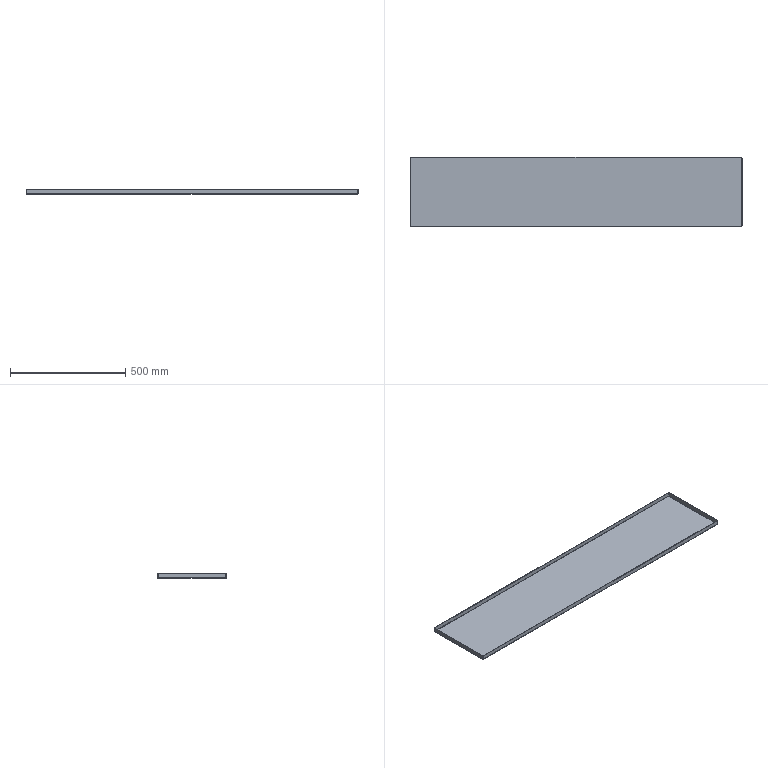Part | STEP file | Part 13 | 1 solid | 38 faces | box 1440 x 300 x 20 mm | volume 983993 mm3 | plane 22 | spline 8 | cylinder 8 | commonest cylinder face diameters 1 x4 5 x4
STEP:
#1=CARTESIAN_POINT('',(-717.5,-147.5,-2.));
#2=VERTEX_POINT('',#1);
#3=CARTESIAN_POINT('',(-717.5,147.5,-2.));
#4=VERTEX_POINT('',#3);
#5=CARTESIAN_POINT('',(-717.5,-147.5,-2.));
#6=DIRECTION('',(0.,1.,0.));
#7=VECTOR('',#6,1000.);
#8=LINE('',#5,#7);
#9=EDGE_CURVE('',#2,#4,#8,.T.);
#10=ORIENTED_EDGE('',*,*,#9,.T.);
#11=CARTESIAN_POINT('',(717.5,147.5,-2.));
#12=VERTEX_POINT('',#11);
#13=CARTESIAN_POINT('',(-717.5,147.5,-2.));
#14=DIRECTION('',(1.,0.,0.));
#15=VECTOR('',#14,1000.);
#16=LINE('',#13,#15);
#17=EDGE_CURVE('',#4,#12,#16,.T.);
#18=ORIENTED_EDGE('',*,*,#17,.T.);
#19=CARTESIAN_POINT('',(717.5,-147.5,-2.));
#20=VERTEX_POINT('',#19);
#21=CARTESIAN_POINT('',(717.5,147.5,-2.));
#22=DIRECTION('',(0.,-1.,0.));
#23=VECTOR('',#22,1000.);
#24=LINE('',#21,#23);
#25=EDGE_CURVE('',#12,#20,#24,.T.);
#26=ORIENTED_EDGE('',*,*,#25,.T.);
#27=CARTESIAN_POINT('',(717.5,-147.5,-2.));
#28=DIRECTION('',(-1.,0.,0.));
#29=VECTOR('',#28,1000.);
#30=LINE('',#27,#29);
#31=EDGE_CURVE('',#20,#2,#30,.T.);
#32=ORIENTED_EDGE('',*,*,#31,.T.);
#33=EDGE_LOOP('',(#10,#18,#26,#32));
#34=FACE_OUTER_BOUND('',#33,.T.);
#35=CARTESIAN_POINT('',(0.,0.,-2.));
#36=DIRECTION('',(0.,0.,1.));
#37=DIRECTION('',(1.,0.,0.));
#38=AXIS2_PLACEMENT_3D('',#35,#36,#37);
#39=PLANE('',#38);
#40=ADVANCED_FACE('',(#34),#39,.F.);
#41=CARTESIAN_POINT('',(-717.5,147.5,0.));
#42=VERTEX_POINT('',#41);
#43=CARTESIAN_POINT('',(717.5,147.5,0.));
#44=VERTEX_POINT('',#43);
#45=CARTESIAN_POINT('',(-717.5,147.5,0.));
#46=DIRECTION('',(1.,0.,0.));
#47=VECTOR('',#46,1000.);
#48=LINE('',#45,#47);
#49=EDGE_CURVE('',#42,#44,#48,.T.);
#50=ORIENTED_EDGE('',*,*,#49,.F.);
#51=CARTESIAN_POINT('',(-717.5,-147.5,0.));
#52=VERTEX_POINT('',#51);
#53=CARTESIAN_POINT('',(-717.5,-147.5,0.));
#54=DIRECTION('',(0.,1.,0.));
#55=VECTOR('',#54,1000.);
#56=LINE('',#53,#55);
#57=EDGE_CURVE('',#52,#42,#56,.T.);
#58=ORIENTED_EDGE('',*,*,#57,.F.);
#59=CARTESIAN_POINT('',(717.5,-147.5,0.));
#60=VERTEX_POINT('',#59);
#61=CARTESIAN_POINT('',(717.5,-147.5,0.));
#62=DIRECTION('',(-1.,0.,0.));
#63=VECTOR('',#62,1000.);
#64=LINE('',#61,#63);
#65=EDGE_CURVE('',#60,#52,#64,.T.);
#66=ORIENTED_EDGE('',*,*,#65,.F.);
#67=CARTESIAN_POINT('',(717.5,147.5,0.));
#68=DIRECTION('',(0.,-1.,0.));
#69=VECTOR('',#68,1000.);
#70=LINE('',#67,#69);
#71=EDGE_CURVE('',#44,#60,#70,.T.);
#72=ORIENTED_EDGE('',*,*,#71,.F.);
#73=EDGE_LOOP('',(#50,#58,#66,#72));
#74=FACE_OUTER_BOUND('',#73,.T.);
#75=CARTESIAN_POINT('',(0.,0.,0.));
#76=DIRECTION('',(0.,0.,1.));
#77=DIRECTION('',(1.,0.,0.));
#78=AXIS2_PLACEMENT_3D('',#75,#76,#77);
#79=PLANE('',#78);
#80=ADVANCED_FACE('',(#74),#79,.T.);
#81=CARTESIAN_POINT('',(717.293,150.,0.5));
#82=VERTEX_POINT('',#81);
#83=CARTESIAN_POINT('',(717.293,148.,0.5));
#84=VERTEX_POINT('',#83);
#85=CARTESIAN_POINT('',(717.293,148.,0.5));
#86=DIRECTION('',(0.,-1.,0.));
#87=VECTOR('',#86,1000.);
#88=LINE('',#85,#87);
#89=EDGE_CURVE('',#82,#84,#88,.T.);
#90=ORIENTED_EDGE('',*,*,#89,.T.);
#91=CARTESIAN_POINT('',(717.5,147.5,0.));
#92=CARTESIAN_POINT('',(717.465,147.631,0.));
#93=CARTESIAN_POINT('',(717.431,147.761,0.05389));
#94=CARTESIAN_POINT('',(717.362,147.946,0.239));
#95=CARTESIAN_POINT('',(717.327,148.,0.3691));
#96=CARTESIAN_POINT('',(717.293,148.,0.5));
#97=B_SPLINE_CURVE_WITH_KNOTS('',3,(#91,#92,#93,#94,#95,#96),.UNSPECIFIED.,.F.,.F.,(4,2,4),(0.,0.5,1.),.UNSPECIFIED.);
#98=EDGE_CURVE('',#44,#84,#97,.T.);
#99=ORIENTED_EDGE('',*,*,#98,.F.);
#100=CARTESIAN_POINT('',(717.5,147.5,0.));
#101=DIRECTION('',(0.,0.,-1.));
#102=VECTOR('',#101,1000.);
#103=LINE('',#100,#102);
#104=EDGE_CURVE('',#44,#12,#103,.T.);
#105=ORIENTED_EDGE('',*,*,#104,.T.);
#106=CARTESIAN_POINT('',(717.5,147.5,-2.));
#107=CARTESIAN_POINT('',(717.483,147.827,-2.));
#108=CARTESIAN_POINT('',(717.465,148.154,-1.935));
#109=CARTESIAN_POINT('',(717.431,148.759,-1.684));
#110=CARTESIAN_POINT('',(717.414,149.036,-1.499));
#111=CARTESIAN_POINT('',(717.379,149.499,-1.036));
#112=CARTESIAN_POINT('',(717.362,149.684,-0.759));
#113=CARTESIAN_POINT('',(717.327,149.935,-0.1544));
#114=CARTESIAN_POINT('',(717.31,150.,0.1728));
#115=CARTESIAN_POINT('',(717.293,150.,0.5));
#116=B_SPLINE_CURVE_WITH_KNOTS('',3,(#106,#107,#108,#109,#110,#111,#112,#113,#114,#115),.UNSPECIFIED.,.F.,.F.,(4,2,2,2,4),(0.,0.25,0.5,0.75,1.),.UNSPECIFIED.);
#117=EDGE_CURVE('',#12,#82,#116,.T.);
#118=ORIENTED_EDGE('',*,*,#117,.T.);
#119=EDGE_LOOP('',(#90,#99,#105,#118));
#120=FACE_OUTER_BOUND('',#119,.T.);
#121=CARTESIAN_POINT('',(717.5,147.5,-2.02));
#122=CARTESIAN_POINT('',(717.483,147.83,-2.02));
#123=CARTESIAN_POINT('',(717.465,148.16,-1.954));
#124=CARTESIAN_POINT('',(717.431,148.769,-1.702));
#125=CARTESIAN_POINT('',(717.414,149.049,-1.515));
#126=CARTESIAN_POINT('',(717.379,149.515,-1.049));
#127=CARTESIAN_POINT('',(717.362,149.702,-0.7691));
#128=CARTESIAN_POINT('',(717.327,149.954,-0.1596));
#129=CARTESIAN_POINT('',(717.31,150.02,0.1701));
#130=CARTESIAN_POINT('',(717.293,150.02,0.5));
#131=CARTESIAN_POINT('',(717.5,147.5,-2.));
#132=CARTESIAN_POINT('',(717.483,147.827,-2.));
#133=CARTESIAN_POINT('',(717.465,148.154,-1.935));
#134=CARTESIAN_POINT('',(717.431,148.759,-1.684));
#135=CARTESIAN_POINT('',(717.414,149.036,-1.499));
#136=CARTESIAN_POINT('',(717.379,149.499,-1.036));
#137=CARTESIAN_POINT('',(717.362,149.684,-0.759));
#138=CARTESIAN_POINT('',(717.327,149.935,-0.1544));
#139=CARTESIAN_POINT('',(717.31,150.,0.1727));
#140=CARTESIAN_POINT('',(717.293,150.,0.5));
#141=CARTESIAN_POINT('',(717.5,147.5,0.));
#142=CARTESIAN_POINT('',(717.483,147.565,0.));
#143=CARTESIAN_POINT('',(717.465,147.631,0.01301));
#144=CARTESIAN_POINT('',(717.431,147.752,0.06311));
#145=CARTESIAN_POINT('',(717.414,147.807,0.1002));
#146=CARTESIAN_POINT('',(717.379,147.9,0.1927));
#147=CARTESIAN_POINT('',(717.362,147.937,0.2482));
#148=CARTESIAN_POINT('',(717.327,147.987,0.3691));
#149=CARTESIAN_POINT('',(717.31,148.,0.4345));
#150=CARTESIAN_POINT('',(717.293,148.,0.5));
#151=CARTESIAN_POINT('',(717.5,147.5,0.0202));
#152=CARTESIAN_POINT('',(717.483,147.563,0.0202));
#153=CARTESIAN_POINT('',(717.465,147.626,0.03269));
#154=CARTESIAN_POINT('',(717.431,147.742,0.08076));
#155=CARTESIAN_POINT('',(717.414,147.795,0.1163));
#156=CARTESIAN_POINT('',(717.379,147.884,0.2051));
#157=CARTESIAN_POINT('',(717.362,147.919,0.2584));
#158=CARTESIAN_POINT('',(717.327,147.967,0.3744));
#159=CARTESIAN_POINT('',(717.31,147.98,0.4372));
#160=CARTESIAN_POINT('',(717.293,147.98,0.5));
#161=B_SPLINE_SURFACE_WITH_KNOTS('',1,3,((#121,#122,#123,#124,#125,#126,#127,#128,#129,#130),(#131,#132,#133,#134,#135,#136,#137,#138,#139,#140),(#141,#142,#143,#144,#145,#146,#147,#148,#149,#150),(#151,#152,#153,#154,#155,#156,#157,#158,#159,#160)),.UNSPECIFIED.,.F.,.F.,.F.,(2,1,1,2),(4,2,2,2,4),(-0.01,0.,1.,1.01),(0.,0.25,0.5,0.75,1.),.UNSPECIFIED.);
#162=ADVANCED_FACE('',(#120),#161,.F.);
#163=CARTESIAN_POINT('',(-717.293,148.,0.5));
#164=VERTEX_POINT('',#163);
#165=CARTESIAN_POINT('',(-717.293,148.,0.5));
#166=CARTESIAN_POINT('',(-717.327,148.,0.3691));
#167=CARTESIAN_POINT('',(-717.362,147.946,0.239));
#168=CARTESIAN_POINT('',(-717.431,147.761,0.05389));
#169=CARTESIAN_POINT('',(-717.465,147.631,0.));
#170=CARTESIAN_POINT('',(-717.5,147.5,0.));
#171=B_SPLINE_CURVE_WITH_KNOTS('',3,(#165,#166,#167,#168,#169,#170),.UNSPECIFIED.,.F.,.F.,(4,2,4),(0.,0.5,1.),.UNSPECIFIED.);
#172=EDGE_CURVE('',#164,#42,#171,.T.);
#173=ORIENTED_EDGE('',*,*,#172,.F.);
#174=CARTESIAN_POINT('',(-717.293,150.,0.5));
#175=VERTEX_POINT('',#174);
#176=CARTESIAN_POINT('',(-717.293,148.,0.5));
#177=DIRECTION('',(0.,-1.,0.));
#178=VECTOR('',#177,1000.);
#179=LINE('',#176,#178);
#180=EDGE_CURVE('',#175,#164,#179,.T.);
#181=ORIENTED_EDGE('',*,*,#180,.F.);
#182=CARTESIAN_POINT('',(-717.293,150.,0.5));
#183=CARTESIAN_POINT('',(-717.31,150.,0.1728));
#184=CARTESIAN_POINT('',(-717.327,149.935,-0.1544));
#185=CARTESIAN_POINT('',(-717.362,149.684,-0.759));
#186=CARTESIAN_POINT('',(-717.379,149.499,-1.036));
#187=CARTESIAN_POINT('',(-717.414,149.036,-1.499));
#188=CARTESIAN_POINT('',(-717.431,148.759,-1.684));
#189=CARTESIAN_POINT('',(-717.465,148.154,-1.935));
#190=CARTESIAN_POINT('',(-717.483,147.827,-2.));
#191=CARTESIAN_POINT('',(-717.5,147.5,-2.));
#192=B_SPLINE_CURVE_WITH_KNOTS('',3,(#182,#183,#184,#185,#186,#187,#188,#189,#190,#191),.UNSPECIFIED.,.F.,.F.,(4,2,2,2,4),(0.,0.25,0.5,0.75,1.),.UNSPECIFIED.);
#193=EDGE_CURVE('',#175,#4,#192,.T.);
#194=ORIENTED_EDGE('',*,*,#193,.T.);
#195=CARTESIAN_POINT('',(-717.5,147.5,0.));
#196=DIRECTION('',(0.,0.,-1.));
#197=VECTOR('',#196,1000.);
#198=LINE('',#195,#197);
#199=EDGE_CURVE('',#42,#4,#198,.T.);
#200=ORIENTED_EDGE('',*,*,#199,.F.);
#201=EDGE_LOOP('',(#173,#181,#194,#200));
#202=FACE_OUTER_BOUND('',#201,.T.);
#203=CARTESIAN_POINT('',(-717.293,150.02,0.5));
#204=CARTESIAN_POINT('',(-717.31,150.02,0.1701));
#205=CARTESIAN_POINT('',(-717.327,149.954,-0.1596));
#206=CARTESIAN_POINT('',(-717.362,149.702,-0.7691));
#207=CARTESIAN_POINT('',(-717.379,149.515,-1.049));
#208=CARTESIAN_POINT('',(-717.414,149.049,-1.515));
#209=CARTESIAN_POINT('',(-717.431,148.769,-1.702));
#210=CARTESIAN_POINT('',(-717.465,148.16,-1.954));
#211=CARTESIAN_POINT('',(-717.483,147.83,-2.02));
#212=CARTESIAN_POINT('',(-717.5,147.5,-2.02));
#213=CARTESIAN_POINT('',(-717.293,150.,0.5));
#214=CARTESIAN_POINT('',(-717.31,150.,0.1727));
#215=CARTESIAN_POINT('',(-717.327,149.935,-0.1544));
#216=CARTESIAN_POINT('',(-717.362,149.684,-0.759));
#217=CARTESIAN_POINT('',(-717.379,149.499,-1.036));
#218=CARTESIAN_POINT('',(-717.414,149.036,-1.499));
#219=CARTESIAN_POINT('',(-717.431,148.759,-1.684));
#220=CARTESIAN_POINT('',(-717.465,148.154,-1.935));
#221=CARTESIAN_POINT('',(-717.483,147.827,-2.));
#222=CARTESIAN_POINT('',(-717.5,147.5,-2.));
#223=CARTESIAN_POINT('',(-717.293,148.,0.5));
#224=CARTESIAN_POINT('',(-717.31,148.,0.4345));
#225=CARTESIAN_POINT('',(-717.327,147.987,0.3691));
#226=CARTESIAN_POINT('',(-717.362,147.937,0.2482));
#227=CARTESIAN_POINT('',(-717.379,147.9,0.1927));
#228=CARTESIAN_POINT('',(-717.414,147.807,0.1002));
#229=CARTESIAN_POINT('',(-717.431,147.752,0.06311));
#230=CARTESIAN_POINT('',(-717.465,147.631,0.01301));
#231=CARTESIAN_POINT('',(-717.483,147.565,0.));
#232=CARTESIAN_POINT('',(-717.5,147.5,0.));
#233=CARTESIAN_POINT('',(-717.293,147.98,0.5));
#234=CARTESIAN_POINT('',(-717.31,147.98,0.4372));
#235=CARTESIAN_POINT('',(-717.327,147.967,0.3744));
#236=CARTESIAN_POINT('',(-717.362,147.919,0.2584));
#237=CARTESIAN_POINT('',(-717.379,147.884,0.2051));
#238=CARTESIAN_POINT('',(-717.414,147.795,0.1163));
#239=CARTESIAN_POINT('',(-717.431,147.742,0.08076));
#240=CARTESIAN_POINT('',(-717.465,147.626,0.03269));
#241=CARTESIAN_POINT('',(-717.483,147.563,0.0202));
#242=CARTESIAN_POINT('',(-717.5,147.5,0.0202));
#243=B_SPLINE_SURFACE_WITH_KNOTS('',1,3,((#203,#204,#205,#206,#207,#208,#209,#210,#211,#212),(#213,#214,#215,#216,#217,#218,#219,#220,#221,#222),(#223,#224,#225,#226,#227,#228,#229,#230,#231,#232),(#233,#234,#235,#236,#237,#238,#239,#240,#241,#242)),.UNSPECIFIED.,.F.,.F.,.F.,(2,1,1,2),(4,2,2,2,4),(-0.01,0.,1.,1.01),(0.,0.25,0.5,0.75,1.),.UNSPECIFIED.);
#244=ADVANCED_FACE('',(#202),#243,.F.);
#245=ORIENTED_EDGE('',*,*,#17,.F.);
#246=ORIENTED_EDGE('',*,*,#193,.F.);
#247=CARTESIAN_POINT('',(0.,150.,0.5));
#248=DIRECTION('',(-1.,0.,0.));
#249=VECTOR('',#248,1000.);
#250=LINE('',#247,#249);
#251=EDGE_CURVE('',#82,#175,#250,.T.);
#252=ORIENTED_EDGE('',*,*,#251,.F.);
#253=ORIENTED_EDGE('',*,*,#117,.F.);
#254=EDGE_LOOP('',(#245,#246,#252,#253));
#255=FACE_OUTER_BOUND('',#254,.T.);
#256=CARTESIAN_POINT('',(-717.5,147.5,0.5));
#257=DIRECTION('',(-1.,0.,0.));
#258=DIRECTION('',(0.,1.,0.));
#259=AXIS2_PLACEMENT_3D('',#256,#257,#258);
#260=CYLINDRICAL_SURFACE('',#259,2.5);
#261=ADVANCED_FACE('',(#255),#260,.T.);
#262=ORIENTED_EDGE('',*,*,#49,.T.);
#263=ORIENTED_EDGE('',*,*,#98,.T.);
#264=CARTESIAN_POINT('',(720.,148.,0.5));
#265=DIRECTION('',(-1.,0.,0.));
#266=VECTOR('',#265,1000.);
#267=LINE('',#264,#266);
#268=EDGE_CURVE('',#84,#164,#267,.T.);
#269=ORIENTED_EDGE('',*,*,#268,.T.);
#270=ORIENTED_EDGE('',*,*,#172,.T.);
#271=EDGE_LOOP('',(#262,#263,#269,#270));
#272=FACE_OUTER_BOUND('',#271,.T.);
#273=CARTESIAN_POINT('',(-717.5,147.5,0.5));
#274=DIRECTION('',(-1.,0.,0.));
#275=DIRECTION('',(0.,1.,0.));
#276=AXIS2_PLACEMENT_3D('',#273,#274,#275);
#277=CYLINDRICAL_SURFACE('',#276,0.5);
#278=ADVANCED_FACE('',(#272),#277,.F.);
#279=CARTESIAN_POINT('',(717.293,148.,18.));
#280=VERTEX_POINT('',#279);
#281=CARTESIAN_POINT('',(717.293,150.,18.));
#282=VERTEX_POINT('',#281);
#283=CARTESIAN_POINT('',(717.293,150.,18.));
#284=DIRECTION('',(0.,1.,0.));
#285=VECTOR('',#284,1000.);
#286=LINE('',#283,#285);
#287=EDGE_CURVE('',#280,#282,#286,.T.);
#288=ORIENTED_EDGE('',*,*,#287,.F.);
#289=CARTESIAN_POINT('',(717.293,148.,0.));
#290=DIRECTION('',(0.,0.,1.));
#291=VECTOR('',#290,1000.);
#292=LINE('',#289,#291);
#293=EDGE_CURVE('',#84,#280,#292,.T.);
#294=ORIENTED_EDGE('',*,*,#293,.F.);
#295=ORIENTED_EDGE('',*,*,#89,.F.);
#296=CARTESIAN_POINT('',(717.293,150.,0.));
#297=DIRECTION('',(0.,0.,-1.));
#298=VECTOR('',#297,1000.);
#299=LINE('',#296,#298);
#300=EDGE_CURVE('',#282,#82,#299,.T.);
#301=ORIENTED_EDGE('',*,*,#300,.F.);
#302=EDGE_LOOP('',(#288,#294,#295,#301));
#303=FACE_OUTER_BOUND('',#302,.T.);
#304=CARTESIAN_POINT('',(717.293,148.,0.));
#305=DIRECTION('',(1.,0.,0.));
#306=DIRECTION('',(0.,0.,-1.));
#307=AXIS2_PLACEMENT_3D('',#304,#305,#306);
#308=PLANE('',#307);
#309=ADVANCED_FACE('',(#303),#308,.T.);
#310=CARTESIAN_POINT('',(-717.293,150.,18.));
#311=VERTEX_POINT('',#310);
#312=CARTESIAN_POINT('',(-717.293,150.,0.));
#313=DIRECTION('',(0.,0.,-1.));
#314=VECTOR('',#313,1000.);
#315=LINE('',#312,#314);
#316=EDGE_CURVE('',#311,#175,#315,.T.);
#317=ORIENTED_EDGE('',*,*,#316,.F.);
#318=CARTESIAN_POINT('',(-720.,150.,18.));
#319=DIRECTION('',(-1.,0.,0.));
#320=VECTOR('',#319,1000.);
#321=LINE('',#318,#320);
#322=EDGE_CURVE('',#282,#311,#321,.T.);
#323=ORIENTED_EDGE('',*,*,#322,.F.);
#324=ORIENTED_EDGE('',*,*,#300,.T.);
#325=ORIENTED_EDGE('',*,*,#251,.T.);
#326=EDGE_LOOP('',(#317,#323,#324,#325));
#327=FACE_OUTER_BOUND('',#326,.T.);
#328=CARTESIAN_POINT('',(0.,150.,0.));
#329=DIRECTION('',(0.,1.,0.));
#330=DIRECTION('',(0.,0.,1.));
#331=AXIS2_PLACEMENT_3D('',#328,#329,#330);
#332=PLANE('',#331);
#333=ADVANCED_FACE('',(#327),#332,.T.);
#334=CARTESIAN_POINT('',(-717.293,148.,18.));
#335=VERTEX_POINT('',#334);
#336=CARTESIAN_POINT('',(0.,148.,18.));
#337=DIRECTION('',(-1.,0.,0.));
#338=VECTOR('',#337,1000.);
#339=LINE('',#336,#338);
#340=EDGE_CURVE('',#280,#335,#339,.T.);
#341=ORIENTED_EDGE('',*,*,#340,.T.);
#342=CARTESIAN_POINT('',(-717.293,148.,0.));
#343=DIRECTION('',(0.,0.,1.));
#344=VECTOR('',#343,1000.);
#345=LINE('',#342,#344);
#346=EDGE_CURVE('',#164,#335,#345,.T.);
#347=ORIENTED_EDGE('',*,*,#346,.F.);
#348=ORIENTED_EDGE('',*,*,#268,.F.);
#349=ORIENTED_EDGE('',*,*,#293,.T.);
#350=EDGE_LOOP('',(#341,#347,#348,#349));
#351=FACE_OUTER_BOUND('',#350,.T.);
#352=CARTESIAN_POINT('',(0.,148.,0.));
#353=DIRECTION('',(0.,1.,0.));
#354=DIRECTION('',(0.,0.,1.));
#355=AXIS2_PLACEMENT_3D('',#352,#353,#354);
#356=PLANE('',#355);
#357=ADVANCED_FACE('',(#351),#356,.F.);
#358=CARTESIAN_POINT('',(-717.293,148.,18.));
#359=DIRECTION('',(0.,1.,0.));
#360=VECTOR('',#359,1000.);
#361=LINE('',#358,#360);
#362=EDGE_CURVE('',#335,#311,#361,.T.);
#363=ORIENTED_EDGE('',*,*,#362,.F.);
#364=ORIENTED_EDGE('',*,*,#340,.F.);
#365=ORIENTED_EDGE('',*,*,#287,.T.);
#366=ORIENTED_EDGE('',*,*,#322,.T.);
#367=EDGE_LOOP('',(#363,#364,#365,#366));
#368=FACE_OUTER_BOUND('',#367,.T.);
#369=CARTESIAN_POINT('',(-720.,150.,18.));
#370=DIRECTION('',(0.,0.,1.));
#371=DIRECTION('',(0.,-1.,0.));
#372=AXIS2_PLACEMENT_3D('',#369,#370,#371);
#373=PLANE('',#372);
#374=ADVANCED_FACE('',(#368),#373,.T.);
#375=ORIENTED_EDGE('',*,*,#346,.T.);
#376=ORIENTED_EDGE('',*,*,#362,.T.);
#377=ORIENTED_EDGE('',*,*,#316,.T.);
#378=ORIENTED_EDGE('',*,*,#180,.T.);
#379=EDGE_LOOP('',(#375,#376,#377,#378));
#380=FACE_OUTER_BOUND('',#379,.T.);
#381=CARTESIAN_POINT('',(-717.293,148.,0.));
#382=DIRECTION('',(1.,0.,0.));
#383=DIRECTION('',(0.,0.,-1.));
#384=AXIS2_PLACEMENT_3D('',#381,#382,#383);
#385=PLANE('',#384);
#386=ADVANCED_FACE('',(#380),#385,.F.);
#387=CARTESIAN_POINT('',(720.,-147.293,0.5));
#388=VERTEX_POINT('',#387);
#389=CARTESIAN_POINT('',(718.,-147.293,0.5));
#390=VERTEX_POINT('',#389);
#391=CARTESIAN_POINT('',(718.,-147.293,0.5));
#392=DIRECTION('',(-1.,0.,0.));
#393=VECTOR('',#392,1000.);
#394=LINE('',#391,#393);
#395=EDGE_CURVE('',#388,#390,#394,.T.);
#396=ORIENTED_EDGE('',*,*,#395,.T.);
#397=CARTESIAN_POINT('',(717.5,-147.5,0.));
#398=CARTESIAN_POINT('',(717.631,-147.465,0.));
#399=CARTESIAN_POINT('',(717.761,-147.431,0.05389));
#400=CARTESIAN_POINT('',(717.946,-147.362,0.239));
#401=CARTESIAN_POINT('',(718.,-147.327,0.3691));
#402=CARTESIAN_POINT('',(718.,-147.293,0.5));
#403=B_SPLINE_CURVE_WITH_KNOTS('',3,(#397,#398,#399,#400,#401,#402),.UNSPECIFIED.,.F.,.F.,(4,2,4),(0.,0.5,1.),.UNSPECIFIED.);
#404=EDGE_CURVE('',#60,#390,#403,.T.);
#405=ORIENTED_EDGE('',*,*,#404,.F.);
#406=CARTESIAN_POINT('',(717.5,-147.5,0.));
#407=DIRECTION('',(0.,0.,-1.));
#408=VECTOR('',#407,1000.);
#409=LINE('',#406,#408);
#410=EDGE_CURVE('',#60,#20,#409,.T.);
#411=ORIENTED_EDGE('',*,*,#410,.T.);
#412=CARTESIAN_POINT('',(717.5,-147.5,-2.));
#413=CARTESIAN_POINT('',(717.827,-147.483,-2.));
#414=CARTESIAN_POINT('',(718.154,-147.465,-1.935));
#415=CARTESIAN_POINT('',(718.759,-147.431,-1.684));
#416=CARTESIAN_POINT('',(719.036,-147.414,-1.499));
#417=CARTESIAN_POINT('',(719.499,-147.379,-1.036));
#418=CARTESIAN_POINT('',(719.684,-147.362,-0.759));
#419=CARTESIAN_POINT('',(719.935,-147.327,-0.1544));
#420=CARTESIAN_POINT('',(720.,-147.31,0.1728));
#421=CARTESIAN_POINT('',(720.,-147.293,0.5));
#422=B_SPLINE_CURVE_WITH_KNOTS('',3,(#412,#413,#414,#415,#416,#417,#418,#419,#420,#421),.UNSPECIFIED.,.F.,.F.,(4,2,2,2,4),(0.,0.25,0.5,0.75,1.),.UNSPECIFIED.);
#423=EDGE_CURVE('',#20,#388,#422,.T.);
#424=ORIENTED_EDGE('',*,*,#423,.T.);
#425=EDGE_LOOP('',(#396,#405,#411,#424));
#426=FACE_OUTER_BOUND('',#425,.T.);
#427=CARTESIAN_POINT('',(717.5,-147.5,-2.02));
#428=CARTESIAN_POINT('',(717.83,-147.483,-2.02));
#429=CARTESIAN_POINT('',(718.16,-147.465,-1.954));
#430=CARTESIAN_POINT('',(718.769,-147.431,-1.702));
#431=CARTESIAN_POINT('',(719.049,-147.414,-1.515));
#432=CARTESIAN_POINT('',(719.515,-147.379,-1.049));
#433=CARTESIAN_POINT('',(719.702,-147.362,-0.7691));
#434=CARTESIAN_POINT('',(719.954,-147.327,-0.1596));
#435=CARTESIAN_POINT('',(720.02,-147.31,0.1701));
#436=CARTESIAN_POINT('',(720.02,-147.293,0.5));
#437=CARTESIAN_POINT('',(717.5,-147.5,-2.));
#438=CARTESIAN_POINT('',(717.827,-147.483,-2.));
#439=CARTESIAN_POINT('',(718.154,-147.465,-1.935));
#440=CARTESIAN_POINT('',(718.759,-147.431,-1.684));
#441=CARTESIAN_POINT('',(719.036,-147.414,-1.499));
#442=CARTESIAN_POINT('',(719.499,-147.379,-1.036));
#443=CARTESIAN_POINT('',(719.684,-147.362,-0.759));
#444=CARTESIAN_POINT('',(719.935,-147.327,-0.1544));
#445=CARTESIAN_POINT('',(720.,-147.31,0.1727));
#446=CARTESIAN_POINT('',(720.,-147.293,0.5));
#447=CARTESIAN_POINT('',(717.5,-147.5,0.));
#448=CARTESIAN_POINT('',(717.565,-147.483,0.));
#449=CARTESIAN_POINT('',(717.631,-147.465,0.01301));
#450=CARTESIAN_POINT('',(717.752,-147.431,0.06311));
#451=CARTESIAN_POINT('',(717.807,-147.414,0.1002));
#452=CARTESIAN_POINT('',(717.9,-147.379,0.1927));
#453=CARTESIAN_POINT('',(717.937,-147.362,0.2482));
#454=CARTESIAN_POINT('',(717.987,-147.327,0.3691));
#455=CARTESIAN_POINT('',(718.,-147.31,0.4345));
#456=CARTESIAN_POINT('',(718.,-147.293,0.5));
#457=CARTESIAN_POINT('',(717.5,-147.5,0.0202));
#458=CARTESIAN_POINT('',(717.563,-147.483,0.0202));
#459=CARTESIAN_POINT('',(717.626,-147.465,0.03269));
#460=CARTESIAN_POINT('',(717.742,-147.431,0.08076));
#461=CARTESIAN_POINT('',(717.795,-147.414,0.1163));
#462=CARTESIAN_POINT('',(717.884,-147.379,0.2051));
#463=CARTESIAN_POINT('',(717.919,-147.362,0.2584));
#464=CARTESIAN_POINT('',(717.967,-147.327,0.3744));
#465=CARTESIAN_POINT('',(717.98,-147.31,0.4372));
#466=CARTESIAN_POINT('',(717.98,-147.293,0.5));
#467=B_SPLINE_SURFACE_WITH_KNOTS('',1,3,((#427,#428,#429,#430,#431,#432,#433,#434,#435,#436),(#437,#438,#439,#440,#441,#442,#443,#444,#445,#446),(#447,#448,#449,#450,#451,#452,#453,#454,#455,#456),(#457,#458,#459,#460,#461,#462,#463,#464,#465,#466)),.UNSPECIFIED.,.F.,.F.,.F.,(2,1,1,2),(4,2,2,2,4),(-0.01,0.,1.,1.01),(0.,0.25,0.5,0.75,1.),.UNSPECIFIED.);
#468=ADVANCED_FACE('',(#426),#467,.F.);
#469=CARTESIAN_POINT('',(718.,147.293,0.5));
#470=VERTEX_POINT('',#469);
#471=CARTESIAN_POINT('',(718.,147.293,0.5));
#472=CARTESIAN_POINT('',(718.,147.327,0.3691));
#473=CARTESIAN_POINT('',(717.946,147.362,0.239));
#474=CARTESIAN_POINT('',(717.761,147.431,0.05389));
#475=CARTESIAN_POINT('',(717.631,147.465,0.));
#476=CARTESIAN_POINT('',(717.5,147.5,0.));
#477=B_SPLINE_CURVE_WITH_KNOTS('',3,(#471,#472,#473,#474,#475,#476),.UNSPECIFIED.,.F.,.F.,(4,2,4),(0.,0.5,1.),.UNSPECIFIED.);
#478=EDGE_CURVE('',#470,#44,#477,.T.);
#479=ORIENTED_EDGE('',*,*,#478,.F.);
#480=CARTESIAN_POINT('',(720.,147.293,0.5));
#481=VERTEX_POINT('',#480);
#482=CARTESIAN_POINT('',(718.,147.293,0.5));
#483=DIRECTION('',(-1.,0.,0.));
#484=VECTOR('',#483,1000.);
#485=LINE('',#482,#484);
#486=EDGE_CURVE('',#481,#470,#485,.T.);
#487=ORIENTED_EDGE('',*,*,#486,.F.);
#488=CARTESIAN_POINT('',(720.,147.293,0.5));
#489=CARTESIAN_POINT('',(720.,147.31,0.1728));
#490=CARTESIAN_POINT('',(719.935,147.327,-0.1544));
#491=CARTESIAN_POINT('',(719.684,147.362,-0.759));
#492=CARTESIAN_POINT('',(719.499,147.379,-1.036));
#493=CARTESIAN_POINT('',(719.036,147.414,-1.499));
#494=CARTESIAN_POINT('',(718.759,147.431,-1.684));
#495=CARTESIAN_POINT('',(718.154,147.465,-1.935));
#496=CARTESIAN_POINT('',(717.827,147.483,-2.));
#497=CARTESIAN_POINT('',(717.5,147.5,-2.));
#498=B_SPLINE_CURVE_WITH_KNOTS('',3,(#488,#489,#490,#491,#492,#493,#494,#495,#496,#497),.UNSPECIFIED.,.F.,.F.,(4,2,2,2,4),(0.,0.25,0.5,0.75,1.),.UNSPECIFIED.);
#499=EDGE_CURVE('',#481,#12,#498,.T.);
#500=ORIENTED_EDGE('',*,*,#499,.T.);
#501=ORIENTED_EDGE('',*,*,#104,.F.);
#502=EDGE_LOOP('',(#479,#487,#500,#501));
#503=FACE_OUTER_BOUND('',#502,.T.);
#504=CARTESIAN_POINT('',(720.02,147.293,0.5));
#505=CARTESIAN_POINT('',(720.02,147.31,0.1701));
#506=CARTESIAN_POINT('',(719.954,147.327,-0.1596));
#507=CARTESIAN_POINT('',(719.702,147.362,-0.7691));
#508=CARTESIAN_POINT('',(719.515,147.379,-1.049));
#509=CARTESIAN_POINT('',(719.049,147.414,-1.515));
#510=CARTESIAN_POINT('',(718.769,147.431,-1.702));
#511=CARTESIAN_POINT('',(718.16,147.465,-1.954));
#512=CARTESIAN_POINT('',(717.83,147.483,-2.02));
#513=CARTESIAN_POINT('',(717.5,147.5,-2.02));
#514=CARTESIAN_POINT('',(720.,147.293,0.5));
#515=CARTESIAN_POINT('',(720.,147.31,0.1727));
#516=CARTESIAN_POINT('',(719.935,147.327,-0.1544));
#517=CARTESIAN_POINT('',(719.684,147.362,-0.759));
#518=CARTESIAN_POINT('',(719.499,147.379,-1.036));
#519=CARTESIAN_POINT('',(719.036,147.414,-1.499));
#520=CARTESIAN_POINT('',(718.759,147.431,-1.684));
#521=CARTESIAN_POINT('',(718.154,147.465,-1.935));
#522=CARTESIAN_POINT('',(717.827,147.483,-2.));
#523=CARTESIAN_POINT('',(717.5,147.5,-2.));
#524=CARTESIAN_POINT('',(718.,147.293,0.5));
#525=CARTESIAN_POINT('',(718.,147.31,0.4345));
#526=CARTESIAN_POINT('',(717.987,147.327,0.3691));
#527=CARTESIAN_POINT('',(717.937,147.362,0.2482));
#528=CARTESIAN_POINT('',(717.9,147.379,0.1927));
#529=CARTESIAN_POINT('',(717.807,147.414,0.1002));
#530=CARTESIAN_POINT('',(717.752,147.431,0.06311));
#531=CARTESIAN_POINT('',(717.631,147.465,0.01301));
#532=CARTESIAN_POINT('',(717.565,147.483,0.));
#533=CARTESIAN_POINT('',(717.5,147.5,0.));
#534=CARTESIAN_POINT('',(717.98,147.293,0.5));
#535=CARTESIAN_POINT('',(717.98,147.31,0.4372));
#536=CARTESIAN_POINT('',(717.967,147.327,0.3744));
#537=CARTESIAN_POINT('',(717.919,147.362,0.2584));
#538=CARTESIAN_POINT('',(717.884,147.379,0.2051));
#539=CARTESIAN_POINT('',(717.795,147.414,0.1163));
#540=CARTESIAN_POINT('',(717.742,147.431,0.08076));
#541=CARTESIAN_POINT('',(717.626,147.465,0.03269));
#542=CARTESIAN_POINT('',(717.563,147.483,0.0202));
#543=CARTESIAN_POINT('',(717.5,147.5,0.0202));
#544=B_SPLINE_SURFACE_WITH_KNOTS('',1,3,((#504,#505,#506,#507,#508,#509,#510,#511,#512,#513),(#514,#515,#516,#517,#518,#519,#520,#521,#522,#523),(#524,#525,#526,#527,#528,#529,#530,#531,#532,#533),(#534,#535,#536,#537,#538,#539,#540,#541,#542,#543)),.UNSPECIFIED.,.F.,.F.,.F.,(2,1,1,2),(4,2,2,2,4),(-0.01,0.,1.,1.01),(0.,0.25,0.5,0.75,1.),.UNSPECIFIED.);
#545=ADVANCED_FACE('',(#503),#544,.F.);
#546=ORIENTED_EDGE('',*,*,#25,.F.);
#547=ORIENTED_EDGE('',*,*,#499,.F.);
#548=CARTESIAN_POINT('',(720.,-150.,0.5));
#549=DIRECTION('',(0.,-1.,0.));
#550=VECTOR('',#549,1000.);
#551=LINE('',#548,#550);
#552=EDGE_CURVE('',#481,#388,#551,.T.);
#553=ORIENTED_EDGE('',*,*,#552,.T.);
#554=ORIENTED_EDGE('',*,*,#423,.F.);
#555=EDGE_LOOP('',(#546,#547,#553,#554));
#556=FACE_OUTER_BOUND('',#555,.T.);
#557=CARTESIAN_POINT('',(717.5,147.5,0.5));
#558=DIRECTION('',(0.,1.,0.));
#559=DIRECTION('',(1.,0.,0.));
#560=AXIS2_PLACEMENT_3D('',#557,#558,#559);
#561=CYLINDRICAL_SURFACE('',#560,2.5);
#562=ADVANCED_FACE('',(#556),#561,.T.);
#563=ORIENTED_EDGE('',*,*,#71,.T.);
#564=ORIENTED_EDGE('',*,*,#404,.T.);
#565=CARTESIAN_POINT('',(718.,-150.,0.5));
#566=DIRECTION('',(0.,1.,0.));
#567=VECTOR('',#566,1000.);
#568=LINE('',#565,#567);
#569=EDGE_CURVE('',#390,#470,#568,.T.);
#570=ORIENTED_EDGE('',*,*,#569,.T.);
#571=ORIENTED_EDGE('',*,*,#478,.T.);
#572=EDGE_LOOP('',(#563,#564,#570,#571));
#573=FACE_OUTER_BOUND('',#572,.T.);
#574=CARTESIAN_POINT('',(717.5,147.5,0.5));
#575=DIRECTION('',(0.,1.,0.));
#576=DIRECTION('',(1.,0.,0.));
#577=AXIS2_PLACEMENT_3D('',#574,#575,#576);
#578=CYLINDRICAL_SURFACE('',#577,0.5);
#579=ADVANCED_FACE('',(#573),#578,.F.);
#580=CARTESIAN_POINT('',(718.,-147.293,18.));
#581=VERTEX_POINT('',#580);
#582=CARTESIAN_POINT('',(720.,-147.293,18.));
#583=VERTEX_POINT('',#582);
#584=CARTESIAN_POINT('',(720.,-147.293,18.));
#585=DIRECTION('',(1.,0.,0.));
#586=VECTOR('',#585,1000.);
#587=LINE('',#584,#586);
#588=EDGE_CURVE('',#581,#583,#587,.T.);
#589=ORIENTED_EDGE('',*,*,#588,.F.);
#590=CARTESIAN_POINT('',(718.,-147.293,0.));
#591=DIRECTION('',(0.,0.,1.));
#592=VECTOR('',#591,1000.);
#593=LINE('',#590,#592);
#594=EDGE_CURVE('',#390,#581,#593,.T.);
#595=ORIENTED_EDGE('',*,*,#594,.F.);
#596=ORIENTED_EDGE('',*,*,#395,.F.);
#597=CARTESIAN_POINT('',(720.,-147.293,0.));
#598=DIRECTION('',(0.,0.,1.));
#599=VECTOR('',#598,1000.);
#600=LINE('',#597,#599);
#601=EDGE_CURVE('',#388,#583,#600,.T.);
#602=ORIENTED_EDGE('',*,*,#601,.T.);
#603=EDGE_LOOP('',(#589,#595,#596,#602));
#604=FACE_OUTER_BOUND('',#603,.T.);
#605=CARTESIAN_POINT('',(718.,-147.293,0.));
#606=DIRECTION('',(0.,-1.,0.));
#607=DIRECTION('',(0.,0.,-1.));
#608=AXIS2_PLACEMENT_3D('',#605,#606,#607);
#609=PLANE('',#608);
#610=ADVANCED_FACE('',(#604),#609,.T.);
#611=ORIENTED_EDGE('',*,*,#552,.F.);
#612=CARTESIAN_POINT('',(720.,147.293,18.));
#613=VERTEX_POINT('',#612);
#614=CARTESIAN_POINT('',(720.,147.293,0.));
#615=DIRECTION('',(0.,0.,1.));
#616=VECTOR('',#615,1000.);
#617=LINE('',#614,#616);
#618=EDGE_CURVE('',#481,#613,#617,.T.);
#619=ORIENTED_EDGE('',*,*,#618,.T.);
#620=CARTESIAN_POINT('',(720.,-150.,18.));
#621=DIRECTION('',(0.,1.,0.));
#622=VECTOR('',#621,1000.);
#623=LINE('',#620,#622);
#624=EDGE_CURVE('',#583,#613,#623,.T.);
#625=ORIENTED_EDGE('',*,*,#624,.F.);
#626=ORIENTED_EDGE('',*,*,#601,.F.);
#627=EDGE_LOOP('',(#611,#619,#625,#626));
#628=FACE_OUTER_BOUND('',#627,.T.);
#629=CARTESIAN_POINT('',(720.,0.,0.));
#630=DIRECTION('',(-1.,0.,0.));
#631=DIRECTION('',(0.,0.,1.));
#632=AXIS2_PLACEMENT_3D('',#629,#630,#631);
#633=PLANE('',#632);
#634=ADVANCED_FACE('',(#628),#633,.F.);
#635=CARTESIAN_POINT('',(718.,147.293,18.));
#636=VERTEX_POINT('',#635);
#637=CARTESIAN_POINT('',(718.,147.293,0.));
#638=DIRECTION('',(0.,0.,1.));
#639=VECTOR('',#638,1000.);
#640=LINE('',#637,#639);
#641=EDGE_CURVE('',#470,#636,#640,.T.);
#642=ORIENTED_EDGE('',*,*,#641,.F.);
#643=ORIENTED_EDGE('',*,*,#569,.F.);
#644=ORIENTED_EDGE('',*,*,#594,.T.);
#645=CARTESIAN_POINT('',(718.,0.,18.));
#646=DIRECTION('',(0.,1.,0.));
#647=VECTOR('',#646,1000.);
#648=LINE('',#645,#647);
#649=EDGE_CURVE('',#581,#636,#648,.T.);
#650=ORIENTED_EDGE('',*,*,#649,.T.);
#651=EDGE_LOOP('',(#642,#643,#644,#650));
#652=FACE_OUTER_BOUND('',#651,.T.);
#653=CARTESIAN_POINT('',(718.,0.,0.));
#654=DIRECTION('',(-1.,0.,0.));
#655=DIRECTION('',(0.,0.,1.));
#656=AXIS2_PLACEMENT_3D('',#653,#654,#655);
#657=PLANE('',#656);
#658=ADVANCED_FACE('',(#652),#657,.T.);
#659=CARTESIAN_POINT('',(718.,147.293,18.));
#660=DIRECTION('',(1.,0.,0.));
#661=VECTOR('',#660,1000.);
#662=LINE('',#659,#661);
#663=EDGE_CURVE('',#636,#613,#662,.T.);
#664=ORIENTED_EDGE('',*,*,#663,.F.);
#665=ORIENTED_EDGE('',*,*,#649,.F.);
#666=ORIENTED_EDGE('',*,*,#588,.T.);
#667=ORIENTED_EDGE('',*,*,#624,.T.);
#668=EDGE_LOOP('',(#664,#665,#666,#667));
#669=FACE_OUTER_BOUND('',#668,.T.);
#670=CARTESIAN_POINT('',(720.,-150.,18.));
#671=DIRECTION('',(0.,0.,1.));
#672=DIRECTION('',(1.,0.,0.));
#673=AXIS2_PLACEMENT_3D('',#670,#671,#672);
#674=PLANE('',#673);
#675=ADVANCED_FACE('',(#669),#674,.T.);
#676=ORIENTED_EDGE('',*,*,#641,.T.);
#677=ORIENTED_EDGE('',*,*,#663,.T.);
#678=ORIENTED_EDGE('',*,*,#618,.F.);
#679=ORIENTED_EDGE('',*,*,#486,.T.);
#680=EDGE_LOOP('',(#676,#677,#678,#679));
#681=FACE_OUTER_BOUND('',#680,.T.);
#682=CARTESIAN_POINT('',(718.,147.293,0.));
#683=DIRECTION('',(0.,-1.,0.));
#684=DIRECTION('',(0.,0.,-1.));
#685=AXIS2_PLACEMENT_3D('',#682,#683,#684);
#686=PLANE('',#685);
#687=ADVANCED_FACE('',(#681),#686,.F.);
#688=CARTESIAN_POINT('',(-717.293,-150.,0.5));
#689=VERTEX_POINT('',#688);
#690=CARTESIAN_POINT('',(-717.293,-148.,0.5));
#691=VERTEX_POINT('',#690);
#692=CARTESIAN_POINT('',(-717.293,-148.,0.5));
#693=DIRECTION('',(0.,1.,0.));
#694=VECTOR('',#693,1000.);
#695=LINE('',#692,#694);
#696=EDGE_CURVE('',#689,#691,#695,.T.);
#697=ORIENTED_EDGE('',*,*,#696,.T.);
#698=CARTESIAN_POINT('',(-717.5,-147.5,0.));
#699=CARTESIAN_POINT('',(-717.465,-147.631,0.));
#700=CARTESIAN_POINT('',(-717.431,-147.761,0.05389));
#701=CARTESIAN_POINT('',(-717.362,-147.946,0.239));
#702=CARTESIAN_POINT('',(-717.327,-148.,0.3691));
#703=CARTESIAN_POINT('',(-717.293,-148.,0.5));
#704=B_SPLINE_CURVE_WITH_KNOTS('',3,(#698,#699,#700,#701,#702,#703),.UNSPECIFIED.,.F.,.F.,(4,2,4),(0.,0.5,1.),.UNSPECIFIED.);
#705=EDGE_CURVE('',#52,#691,#704,.T.);
#706=ORIENTED_EDGE('',*,*,#705,.F.);
#707=CARTESIAN_POINT('',(-717.5,-147.5,0.));
#708=DIRECTION('',(0.,0.,-1.));
#709=VECTOR('',#708,1000.);
#710=LINE('',#707,#709);
#711=EDGE_CURVE('',#52,#2,#710,.T.);
#712=ORIENTED_EDGE('',*,*,#711,.T.);
#713=CARTESIAN_POINT('',(-717.5,-147.5,-2.));
#714=CARTESIAN_POINT('',(-717.483,-147.827,-2.));
#715=CARTESIAN_POINT('',(-717.465,-148.154,-1.935));
#716=CARTESIAN_POINT('',(-717.431,-148.759,-1.684));
#717=CARTESIAN_POINT('',(-717.414,-149.036,-1.499));
#718=CARTESIAN_POINT('',(-717.379,-149.499,-1.036));
#719=CARTESIAN_POINT('',(-717.362,-149.684,-0.759));
#720=CARTESIAN_POINT('',(-717.327,-149.935,-0.1544));
#721=CARTESIAN_POINT('',(-717.31,-150.,0.1728));
#722=CARTESIAN_POINT('',(-717.293,-150.,0.5));
#723=B_SPLINE_CURVE_WITH_KNOTS('',3,(#713,#714,#715,#716,#717,#718,#719,#720,#721,#722),.UNSPECIFIED.,.F.,.F.,(4,2,2,2,4),(0.,0.25,0.5,0.75,1.),.UNSPECIFIED.);
#724=EDGE_CURVE('',#2,#689,#723,.T.);
#725=ORIENTED_EDGE('',*,*,#724,.T.);
#726=EDGE_LOOP('',(#697,#706,#712,#725));
#727=FACE_OUTER_BOUND('',#726,.T.);
#728=CARTESIAN_POINT('',(-717.5,-147.5,-2.02));
#729=CARTESIAN_POINT('',(-717.483,-147.83,-2.02));
#730=CARTESIAN_POINT('',(-717.465,-148.16,-1.954));
#731=CARTESIAN_POINT('',(-717.431,-148.769,-1.702));
#732=CARTESIAN_POINT('',(-717.414,-149.049,-1.515));
#733=CARTESIAN_POINT('',(-717.379,-149.515,-1.049));
#734=CARTESIAN_POINT('',(-717.362,-149.702,-0.7691));
#735=CARTESIAN_POINT('',(-717.327,-149.954,-0.1596));
#736=CARTESIAN_POINT('',(-717.31,-150.02,0.1701));
#737=CARTESIAN_POINT('',(-717.293,-150.02,0.5));
#738=CARTESIAN_POINT('',(-717.5,-147.5,-2.));
#739=CARTESIAN_POINT('',(-717.483,-147.827,-2.));
#740=CARTESIAN_POINT('',(-717.465,-148.154,-1.935));
#741=CARTESIAN_POINT('',(-717.431,-148.759,-1.684));
#742=CARTESIAN_POINT('',(-717.414,-149.036,-1.499));
#743=CARTESIAN_POINT('',(-717.379,-149.499,-1.036));
#744=CARTESIAN_POINT('',(-717.362,-149.684,-0.759));
#745=CARTESIAN_POINT('',(-717.327,-149.935,-0.1544));
#746=CARTESIAN_POINT('',(-717.31,-150.,0.1727));
#747=CARTESIAN_POINT('',(-717.293,-150.,0.5));
#748=CARTESIAN_POINT('',(-717.5,-147.5,0.));
#749=CARTESIAN_POINT('',(-717.483,-147.565,0.));
#750=CARTESIAN_POINT('',(-717.465,-147.631,0.01301));
#751=CARTESIAN_POINT('',(-717.431,-147.752,0.06311));
#752=CARTESIAN_POINT('',(-717.414,-147.807,0.1002));
#753=CARTESIAN_POINT('',(-717.379,-147.9,0.1927));
#754=CARTESIAN_POINT('',(-717.362,-147.937,0.2482));
#755=CARTESIAN_POINT('',(-717.327,-147.987,0.3691));
#756=CARTESIAN_POINT('',(-717.31,-148.,0.4345));
#757=CARTESIAN_POINT('',(-717.293,-148.,0.5));
#758=CARTESIAN_POINT('',(-717.5,-147.5,0.0202));
#759=CARTESIAN_POINT('',(-717.483,-147.563,0.0202));
#760=CARTESIAN_POINT('',(-717.465,-147.626,0.03269));
#761=CARTESIAN_POINT('',(-717.431,-147.742,0.08076));
#762=CARTESIAN_POINT('',(-717.414,-147.795,0.1163));
#763=CARTESIAN_POINT('',(-717.379,-147.884,0.2051));
#764=CARTESIAN_POINT('',(-717.362,-147.919,0.2584));
#765=CARTESIAN_POINT('',(-717.327,-147.967,0.3744));
#766=CARTESIAN_POINT('',(-717.31,-147.98,0.4372));
#767=CARTESIAN_POINT('',(-717.293,-147.98,0.5));
#768=B_SPLINE_SURFACE_WITH_KNOTS('',1,3,((#728,#729,#730,#731,#732,#733,#734,#735,#736,#737),(#738,#739,#740,#741,#742,#743,#744,#745,#746,#747),(#748,#749,#750,#751,#752,#753,#754,#755,#756,#757),(#758,#759,#760,#761,#762,#763,#764,#765,#766,#767)),.UNSPECIFIED.,.F.,.F.,.F.,(2,1,1,2),(4,2,2,2,4),(-0.01,0.,1.,1.01),(0.,0.25,0.5,0.75,1.),.UNSPECIFIED.);
#769=ADVANCED_FACE('',(#727),#768,.F.);
#770=CARTESIAN_POINT('',(717.293,-148.,0.5));
#771=VERTEX_POINT('',#770);
#772=CARTESIAN_POINT('',(717.293,-148.,0.5));
#773=CARTESIAN_POINT('',(717.327,-148.,0.3691));
#774=CARTESIAN_POINT('',(717.362,-147.946,0.239));
#775=CARTESIAN_POINT('',(717.431,-147.761,0.05389));
#776=CARTESIAN_POINT('',(717.465,-147.631,0.));
#777=CARTESIAN_POINT('',(717.5,-147.5,0.));
#778=B_SPLINE_CURVE_WITH_KNOTS('',3,(#772,#773,#774,#775,#776,#777),.UNSPECIFIED.,.F.,.F.,(4,2,4),(0.,0.5,1.),.UNSPECIFIED.);
#779=EDGE_CURVE('',#771,#60,#778,.T.);
#780=ORIENTED_EDGE('',*,*,#779,.F.);
#781=CARTESIAN_POINT('',(717.293,-150.,0.5));
#782=VERTEX_POINT('',#781);
#783=CARTESIAN_POINT('',(717.293,-148.,0.5));
#784=DIRECTION('',(0.,1.,0.));
#785=VECTOR('',#784,1000.);
#786=LINE('',#783,#785);
#787=EDGE_CURVE('',#782,#771,#786,.T.);
#788=ORIENTED_EDGE('',*,*,#787,.F.);
#789=CARTESIAN_POINT('',(717.293,-150.,0.5));
#790=CARTESIAN_POINT('',(717.31,-150.,0.1728));
#791=CARTESIAN_POINT('',(717.327,-149.935,-0.1544));
#792=CARTESIAN_POINT('',(717.362,-149.684,-0.759));
#793=CARTESIAN_POINT('',(717.379,-149.499,-1.036));
#794=CARTESIAN_POINT('',(717.414,-149.036,-1.499));
#795=CARTESIAN_POINT('',(717.431,-148.759,-1.684));
#796=CARTESIAN_POINT('',(717.465,-148.154,-1.935));
#797=CARTESIAN_POINT('',(717.483,-147.827,-2.));
#798=CARTESIAN_POINT('',(717.5,-147.5,-2.));
#799=B_SPLINE_CURVE_WITH_KNOTS('',3,(#789,#790,#791,#792,#793,#794,#795,#796,#797,#798),.UNSPECIFIED.,.F.,.F.,(4,2,2,2,4),(0.,0.25,0.5,0.75,1.),.UNSPECIFIED.);
#800=EDGE_CURVE('',#782,#20,#799,.T.);
#801=ORIENTED_EDGE('',*,*,#800,.T.);
#802=ORIENTED_EDGE('',*,*,#410,.F.);
#803=EDGE_LOOP('',(#780,#788,#801,#802));
#804=FACE_OUTER_BOUND('',#803,.T.);
#805=CARTESIAN_POINT('',(717.293,-150.02,0.5));
#806=CARTESIAN_POINT('',(717.31,-150.02,0.1701));
#807=CARTESIAN_POINT('',(717.327,-149.954,-0.1596));
#808=CARTESIAN_POINT('',(717.362,-149.702,-0.7691));
#809=CARTESIAN_POINT('',(717.379,-149.515,-1.049));
#810=CARTESIAN_POINT('',(717.414,-149.049,-1.515));
#811=CARTESIAN_POINT('',(717.431,-148.769,-1.702));
#812=CARTESIAN_POINT('',(717.465,-148.16,-1.954));
#813=CARTESIAN_POINT('',(717.483,-147.83,-2.02));
#814=CARTESIAN_POINT('',(717.5,-147.5,-2.02));
#815=CARTESIAN_POINT('',(717.293,-150.,0.5));
#816=CARTESIAN_POINT('',(717.31,-150.,0.1727));
#817=CARTESIAN_POINT('',(717.327,-149.935,-0.1544));
#818=CARTESIAN_POINT('',(717.362,-149.684,-0.759));
#819=CARTESIAN_POINT('',(717.379,-149.499,-1.036));
#820=CARTESIAN_POINT('',(717.414,-149.036,-1.499));
#821=CARTESIAN_POINT('',(717.431,-148.759,-1.684));
#822=CARTESIAN_POINT('',(717.465,-148.154,-1.935));
#823=CARTESIAN_POINT('',(717.483,-147.827,-2.));
#824=CARTESIAN_POINT('',(717.5,-147.5,-2.));
#825=CARTESIAN_POINT('',(717.293,-148.,0.5));
#826=CARTESIAN_POINT('',(717.31,-148.,0.4345));
#827=CARTESIAN_POINT('',(717.327,-147.987,0.3691));
#828=CARTESIAN_POINT('',(717.362,-147.937,0.2482));
#829=CARTESIAN_POINT('',(717.379,-147.9,0.1927));
#830=CARTESIAN_POINT('',(717.414,-147.807,0.1002));
#831=CARTESIAN_POINT('',(717.431,-147.752,0.06311));
#832=CARTESIAN_POINT('',(717.465,-147.631,0.01301));
#833=CARTESIAN_POINT('',(717.483,-147.565,0.));
#834=CARTESIAN_POINT('',(717.5,-147.5,0.));
#835=CARTESIAN_POINT('',(717.293,-147.98,0.5));
#836=CARTESIAN_POINT('',(717.31,-147.98,0.4372));
#837=CARTESIAN_POINT('',(717.327,-147.967,0.3744));
#838=CARTESIAN_POINT('',(717.362,-147.919,0.2584));
#839=CARTESIAN_POINT('',(717.379,-147.884,0.2051));
#840=CARTESIAN_POINT('',(717.414,-147.795,0.1163));
#841=CARTESIAN_POINT('',(717.431,-147.742,0.08076));
#842=CARTESIAN_POINT('',(717.465,-147.626,0.03269));
#843=CARTESIAN_POINT('',(717.483,-147.563,0.0202));
#844=CARTESIAN_POINT('',(717.5,-147.5,0.0202));
#845=B_SPLINE_SURFACE_WITH_KNOTS('',1,3,((#805,#806,#807,#808,#809,#810,#811,#812,#813,#814),(#815,#816,#817,#818,#819,#820,#821,#822,#823,#824),(#825,#826,#827,#828,#829,#830,#831,#832,#833,#834),(#835,#836,#837,#838,#839,#840,#841,#842,#843,#844)),.UNSPECIFIED.,.F.,.F.,.F.,(2,1,1,2),(4,2,2,2,4),(-0.01,0.,1.,1.01),(0.,0.25,0.5,0.75,1.),.UNSPECIFIED.);
#846=ADVANCED_FACE('',(#804),#845,.F.);
#847=ORIENTED_EDGE('',*,*,#31,.F.);
#848=ORIENTED_EDGE('',*,*,#800,.F.);
#849=CARTESIAN_POINT('',(-720.,-150.,0.5));
#850=DIRECTION('',(-1.,0.,0.));
#851=VECTOR('',#850,1000.);
#852=LINE('',#849,#851);
#853=EDGE_CURVE('',#782,#689,#852,.T.);
#854=ORIENTED_EDGE('',*,*,#853,.T.);
#855=ORIENTED_EDGE('',*,*,#724,.F.);
#856=EDGE_LOOP('',(#847,#848,#854,#855));
#857=FACE_OUTER_BOUND('',#856,.T.);
#858=CARTESIAN_POINT('',(717.5,-147.5,0.5));
#859=DIRECTION('',(1.,0.,0.));
#860=DIRECTION('',(0.,-1.,0.));
#861=AXIS2_PLACEMENT_3D('',#858,#859,#860);
#862=CYLINDRICAL_SURFACE('',#861,2.5);
#863=ADVANCED_FACE('',(#857),#862,.T.);
#864=ORIENTED_EDGE('',*,*,#65,.T.);
#865=ORIENTED_EDGE('',*,*,#705,.T.);
#866=CARTESIAN_POINT('',(-720.,-148.,0.5));
#867=DIRECTION('',(1.,0.,0.));
#868=VECTOR('',#867,1000.);
#869=LINE('',#866,#868);
#870=EDGE_CURVE('',#691,#771,#869,.T.);
#871=ORIENTED_EDGE('',*,*,#870,.T.);
#872=ORIENTED_EDGE('',*,*,#779,.T.);
#873=EDGE_LOOP('',(#864,#865,#871,#872));
#874=FACE_OUTER_BOUND('',#873,.T.);
#875=CARTESIAN_POINT('',(717.5,-147.5,0.5));
#876=DIRECTION('',(1.,0.,0.));
#877=DIRECTION('',(0.,-1.,0.));
#878=AXIS2_PLACEMENT_3D('',#875,#876,#877);
#879=CYLINDRICAL_SURFACE('',#878,0.5);
#880=ADVANCED_FACE('',(#874),#879,.F.);
#881=CARTESIAN_POINT('',(-717.293,-148.,18.));
#882=VERTEX_POINT('',#881);
#883=CARTESIAN_POINT('',(-717.293,-150.,18.));
#884=VERTEX_POINT('',#883);
#885=CARTESIAN_POINT('',(-717.293,-150.,18.));
#886=DIRECTION('',(0.,-1.,0.));
#887=VECTOR('',#886,1000.);
#888=LINE('',#885,#887);
#889=EDGE_CURVE('',#882,#884,#888,.T.);
#890=ORIENTED_EDGE('',*,*,#889,.F.);
#891=CARTESIAN_POINT('',(-717.293,-148.,0.));
#892=DIRECTION('',(0.,0.,1.));
#893=VECTOR('',#892,1000.);
#894=LINE('',#891,#893);
#895=EDGE_CURVE('',#691,#882,#894,.T.);
#896=ORIENTED_EDGE('',*,*,#895,.F.);
#897=ORIENTED_EDGE('',*,*,#696,.F.);
#898=CARTESIAN_POINT('',(-717.293,-150.,0.));
#899=DIRECTION('',(0.,0.,1.));
#900=VECTOR('',#899,1000.);
#901=LINE('',#898,#900);
#902=EDGE_CURVE('',#689,#884,#901,.T.);
#903=ORIENTED_EDGE('',*,*,#902,.T.);
#904=EDGE_LOOP('',(#890,#896,#897,#903));
#905=FACE_OUTER_BOUND('',#904,.T.);
#906=CARTESIAN_POINT('',(-717.293,-148.,0.));
#907=DIRECTION('',(-1.,0.,0.));
#908=DIRECTION('',(0.,0.,1.));
#909=AXIS2_PLACEMENT_3D('',#906,#907,#908);
#910=PLANE('',#909);
#911=ADVANCED_FACE('',(#905),#910,.T.);
#912=ORIENTED_EDGE('',*,*,#853,.F.);
#913=CARTESIAN_POINT('',(717.293,-150.,18.));
#914=VERTEX_POINT('',#913);
#915=CARTESIAN_POINT('',(717.293,-150.,0.));
#916=DIRECTION('',(0.,0.,1.));
#917=VECTOR('',#916,1000.);
#918=LINE('',#915,#917);
#919=EDGE_CURVE('',#782,#914,#918,.T.);
#920=ORIENTED_EDGE('',*,*,#919,.T.);
#921=CARTESIAN_POINT('',(-720.,-150.,18.));
#922=DIRECTION('',(1.,0.,0.));
#923=VECTOR('',#922,1000.);
#924=LINE('',#921,#923);
#925=EDGE_CURVE('',#884,#914,#924,.T.);
#926=ORIENTED_EDGE('',*,*,#925,.F.);
#927=ORIENTED_EDGE('',*,*,#902,.F.);
#928=EDGE_LOOP('',(#912,#920,#926,#927));
#929=FACE_OUTER_BOUND('',#928,.T.);
#930=CARTESIAN_POINT('',(0.,-150.,0.));
#931=DIRECTION('',(0.,1.,0.));
#932=DIRECTION('',(0.,0.,1.));
#933=AXIS2_PLACEMENT_3D('',#930,#931,#932);
#934=PLANE('',#933);
#935=ADVANCED_FACE('',(#929),#934,.F.);
#936=CARTESIAN_POINT('',(717.293,-148.,18.));
#937=VERTEX_POINT('',#936);
#938=CARTESIAN_POINT('',(717.293,-148.,0.));
#939=DIRECTION('',(0.,0.,1.));
#940=VECTOR('',#939,1000.);
#941=LINE('',#938,#940);
#942=EDGE_CURVE('',#771,#937,#941,.T.);
#943=ORIENTED_EDGE('',*,*,#942,.F.);
#944=ORIENTED_EDGE('',*,*,#870,.F.);
#945=ORIENTED_EDGE('',*,*,#895,.T.);
#946=CARTESIAN_POINT('',(0.,-148.,18.));
#947=DIRECTION('',(1.,0.,0.));
#948=VECTOR('',#947,1000.);
#949=LINE('',#946,#948);
#950=EDGE_CURVE('',#882,#937,#949,.T.);
#951=ORIENTED_EDGE('',*,*,#950,.T.);
#952=EDGE_LOOP('',(#943,#944,#945,#951));
#953=FACE_OUTER_BOUND('',#952,.T.);
#954=CARTESIAN_POINT('',(0.,-148.,0.));
#955=DIRECTION('',(0.,1.,0.));
#956=DIRECTION('',(0.,0.,1.));
#957=AXIS2_PLACEMENT_3D('',#954,#955,#956);
#958=PLANE('',#957);
#959=ADVANCED_FACE('',(#953),#958,.T.);
#960=CARTESIAN_POINT('',(717.293,-148.,18.));
#961=DIRECTION('',(0.,-1.,0.));
#962=VECTOR('',#961,1000.);
#963=LINE('',#960,#962);
#964=EDGE_CURVE('',#937,#914,#963,.T.);
#965=ORIENTED_EDGE('',*,*,#964,.F.);
#966=ORIENTED_EDGE('',*,*,#950,.F.);
#967=ORIENTED_EDGE('',*,*,#889,.T.);
#968=ORIENTED_EDGE('',*,*,#925,.T.);
#969=EDGE_LOOP('',(#965,#966,#967,#968));
#970=FACE_OUTER_BOUND('',#969,.T.);
#971=CARTESIAN_POINT('',(-720.,-150.,18.));
#972=DIRECTION('',(0.,0.,1.));
#973=DIRECTION('',(0.,-1.,0.));
#974=AXIS2_PLACEMENT_3D('',#971,#972,#973);
#975=PLANE('',#974);
#976=ADVANCED_FACE('',(#970),#975,.T.);
#977=ORIENTED_EDGE('',*,*,#942,.T.);
#978=ORIENTED_EDGE('',*,*,#964,.T.);
#979=ORIENTED_EDGE('',*,*,#919,.F.);
#980=ORIENTED_EDGE('',*,*,#787,.T.);
#981=EDGE_LOOP('',(#977,#978,#979,#980));
#982=FACE_OUTER_BOUND('',#981,.T.);
#983=CARTESIAN_POINT('',(717.293,-148.,0.));
#984=DIRECTION('',(-1.,0.,0.));
#985=DIRECTION('',(0.,0.,1.));
#986=AXIS2_PLACEMENT_3D('',#983,#984,#985);
#987=PLANE('',#986);
#988=ADVANCED_FACE('',(#982),#987,.F.);
#989=CARTESIAN_POINT('',(-720.,147.293,0.5));
#990=VERTEX_POINT('',#989);
#991=CARTESIAN_POINT('',(-718.,147.293,0.5));
#992=VERTEX_POINT('',#991);
#993=CARTESIAN_POINT('',(-718.,147.293,0.5));
#994=DIRECTION('',(1.,0.,0.));
#995=VECTOR('',#994,1000.);
#996=LINE('',#993,#995);
#997=EDGE_CURVE('',#990,#992,#996,.T.);
#998=ORIENTED_EDGE('',*,*,#997,.T.);
#999=CARTESIAN_POINT('',(-717.5,147.5,0.));
#1000=CARTESIAN_POINT('',(-717.631,147.465,0.));
#1001=CARTESIAN_POINT('',(-717.761,147.431,0.05389));
#1002=CARTESIAN_POINT('',(-717.946,147.362,0.239));
#1003=CARTESIAN_POINT('',(-718.,147.327,0.3691));
#1004=CARTESIAN_POINT('',(-718.,147.293,0.5));
#1005=B_SPLINE_CURVE_WITH_KNOTS('',3,(#999,#1000,#1001,#1002,#1003,#1004),.UNSPECIFIED.,.F.,.F.,(4,2,4),(0.,0.5,1.),.UNSPECIFIED.);
#1006=EDGE_CURVE('',#42,#992,#1005,.T.);
#1007=ORIENTED_EDGE('',*,*,#1006,.F.);
#1008=ORIENTED_EDGE('',*,*,#199,.T.);
#1009=CARTESIAN_POINT('',(-717.5,147.5,-2.));
#1010=CARTESIAN_POINT('',(-717.827,147.483,-2.));
#1011=CARTESIAN_POINT('',(-718.154,147.465,-1.935));
#1012=CARTESIAN_POINT('',(-718.759,147.431,-1.684));
#1013=CARTESIAN_POINT('',(-719.036,147.414,-1.499));
#1014=CARTESIAN_POINT('',(-719.499,147.379,-1.036));
#1015=CARTESIAN_POINT('',(-719.684,147.362,-0.759));
#1016=CARTESIAN_POINT('',(-719.935,147.327,-0.1544));
#1017=CARTESIAN_POINT('',(-720.,147.31,0.1728));
#1018=CARTESIAN_POINT('',(-720.,147.293,0.5));
#1019=B_SPLINE_CURVE_WITH_KNOTS('',3,(#1009,#1010,#1011,#1012,#1013,#1014,#1015,#1016,#1017,#1018),.UNSPECIFIED.,.F.,.F.,(4,2,2,2,4),(0.,0.25,0.5,0.75,1.),.UNSPECIFIED.);
#1020=EDGE_CURVE('',#4,#990,#1019,.T.);
#1021=ORIENTED_EDGE('',*,*,#1020,.T.);
#1022=EDGE_LOOP('',(#998,#1007,#1008,#1021));
#1023=FACE_OUTER_BOUND('',#1022,.T.);
#1024=CARTESIAN_POINT('',(-717.5,147.5,-2.02));
#1025=CARTESIAN_POINT('',(-717.83,147.483,-2.02));
#1026=CARTESIAN_POINT('',(-718.16,147.465,-1.954));
#1027=CARTESIAN_POINT('',(-718.769,147.431,-1.702));
#1028=CARTESIAN_POINT('',(-719.049,147.414,-1.515));
#1029=CARTESIAN_POINT('',(-719.515,147.379,-1.049));
#1030=CARTESIAN_POINT('',(-719.702,147.362,-0.7691));
#1031=CARTESIAN_POINT('',(-719.954,147.327,-0.1596));
#1032=CARTESIAN_POINT('',(-720.02,147.31,0.1701));
#1033=CARTESIAN_POINT('',(-720.02,147.293,0.5));
#1034=CARTESIAN_POINT('',(-717.5,147.5,-2.));
#1035=CARTESIAN_POINT('',(-717.827,147.483,-2.));
#1036=CARTESIAN_POINT('',(-718.154,147.465,-1.935));
#1037=CARTESIAN_POINT('',(-718.759,147.431,-1.684));
#1038=CARTESIAN_POINT('',(-719.036,147.414,-1.499));
#1039=CARTESIAN_POINT('',(-719.499,147.379,-1.036));
#1040=CARTESIAN_POINT('',(-719.684,147.362,-0.759));
#1041=CARTESIAN_POINT('',(-719.935,147.327,-0.1544));
#1042=CARTESIAN_POINT('',(-720.,147.31,0.1727));
#1043=CARTESIAN_POINT('',(-720.,147.293,0.5));
#1044=CARTESIAN_POINT('',(-717.5,147.5,0.));
#1045=CARTESIAN_POINT('',(-717.565,147.483,0.));
#1046=CARTESIAN_POINT('',(-717.631,147.465,0.01301));
#1047=CARTESIAN_POINT('',(-717.752,147.431,0.06311));
#1048=CARTESIAN_POINT('',(-717.807,147.414,0.1002));
#1049=CARTESIAN_POINT('',(-717.9,147.379,0.1927));
#1050=CARTESIAN_POINT('',(-717.937,147.362,0.2482));
#1051=CARTESIAN_POINT('',(-717.987,147.327,0.3691));
#1052=CARTESIAN_POINT('',(-718.,147.31,0.4345));
#1053=CARTESIAN_POINT('',(-718.,147.293,0.5));
#1054=CARTESIAN_POINT('',(-717.5,147.5,0.0202));
#1055=CARTESIAN_POINT('',(-717.563,147.483,0.0202));
#1056=CARTESIAN_POINT('',(-717.626,147.465,0.03269));
#1057=CARTESIAN_POINT('',(-717.742,147.431,0.08076));
#1058=CARTESIAN_POINT('',(-717.795,147.414,0.1163));
#1059=CARTESIAN_POINT('',(-717.884,147.379,0.2051));
#1060=CARTESIAN_POINT('',(-717.919,147.362,0.2584));
#1061=CARTESIAN_POINT('',(-717.967,147.327,0.3744));
#1062=CARTESIAN_POINT('',(-717.98,147.31,0.4372));
#1063=CARTESIAN_POINT('',(-717.98,147.293,0.5));
#1064=B_SPLINE_SURFACE_WITH_KNOTS('',1,3,((#1024,#1025,#1026,#1027,#1028,#1029,#1030,#1031,#1032,#1033),(#1034,#1035,#1036,#1037,#1038,#1039,#1040,#1041,#1042,#1043),(#1044,#1045,#1046,#1047,#1048,#1049,#1050,#1051,#1052,#1053),(#1054,#1055,#1056,#1057,#1058,#1059,#1060,#1061,#1062,#1063)),.UNSPECIFIED.,.F.,.F.,.F.,(2,1,1,2),(4,2,2,2,4),(-0.01,0.,1.,1.01),(0.,0.25,0.5,0.75,1.),.UNSPECIFIED.);
#1065=ADVANCED_FACE('',(#1023),#1064,.F.);
#1066=CARTESIAN_POINT('',(-718.,-147.293,0.5));
#1067=VERTEX_POINT('',#1066);
#1068=CARTESIAN_POINT('',(-718.,-147.293,0.5));
#1069=CARTESIAN_POINT('',(-718.,-147.327,0.3691));
#1070=CARTESIAN_POINT('',(-717.946,-147.362,0.239));
#1071=CARTESIAN_POINT('',(-717.761,-147.431,0.05389));
#1072=CARTESIAN_POINT('',(-717.631,-147.465,0.));
#1073=CARTESIAN_POINT('',(-717.5,-147.5,0.));
#1074=B_SPLINE_CURVE_WITH_KNOTS('',3,(#1068,#1069,#1070,#1071,#1072,#1073),.UNSPECIFIED.,.F.,.F.,(4,2,4),(0.,0.5,1.),.UNSPECIFIED.);
#1075=EDGE_CURVE('',#1067,#52,#1074,.T.);
#1076=ORIENTED_EDGE('',*,*,#1075,.F.);
#1077=CARTESIAN_POINT('',(-720.,-147.293,0.5));
#1078=VERTEX_POINT('',#1077);
#1079=CARTESIAN_POINT('',(-718.,-147.293,0.5));
#1080=DIRECTION('',(1.,0.,0.));
#1081=VECTOR('',#1080,1000.);
#1082=LINE('',#1079,#1081);
#1083=EDGE_CURVE('',#1078,#1067,#1082,.T.);
#1084=ORIENTED_EDGE('',*,*,#1083,.F.);
#1085=CARTESIAN_POINT('',(-720.,-147.293,0.5));
#1086=CARTESIAN_POINT('',(-720.,-147.31,0.1728));
#1087=CARTESIAN_POINT('',(-719.935,-147.327,-0.1544));
#1088=CARTESIAN_POINT('',(-719.684,-147.362,-0.759));
#1089=CARTESIAN_POINT('',(-719.499,-147.379,-1.036));
#1090=CARTESIAN_POINT('',(-719.036,-147.414,-1.499));
#1091=CARTESIAN_POINT('',(-718.759,-147.431,-1.684));
#1092=CARTESIAN_POINT('',(-718.154,-147.465,-1.935));
#1093=CARTESIAN_POINT('',(-717.827,-147.483,-2.));
#1094=CARTESIAN_POINT('',(-717.5,-147.5,-2.));
#1095=B_SPLINE_CURVE_WITH_KNOTS('',3,(#1085,#1086,#1087,#1088,#1089,#1090,#1091,#1092,#1093,#1094),.UNSPECIFIED.,.F.,.F.,(4,2,2,2,4),(0.,0.25,0.5,0.75,1.),.UNSPECIFIED.);
#1096=EDGE_CURVE('',#1078,#2,#1095,.T.);
#1097=ORIENTED_EDGE('',*,*,#1096,.T.);
#1098=ORIENTED_EDGE('',*,*,#711,.F.);
#1099=EDGE_LOOP('',(#1076,#1084,#1097,#1098));
#1100=FACE_OUTER_BOUND('',#1099,.T.);
#1101=CARTESIAN_POINT('',(-720.02,-147.293,0.5));
#1102=CARTESIAN_POINT('',(-720.02,-147.31,0.1701));
#1103=CARTESIAN_POINT('',(-719.954,-147.327,-0.1596));
#1104=CARTESIAN_POINT('',(-719.702,-147.362,-0.7691));
#1105=CARTESIAN_POINT('',(-719.515,-147.379,-1.049));
#1106=CARTESIAN_POINT('',(-719.049,-147.414,-1.515));
#1107=CARTESIAN_POINT('',(-718.769,-147.431,-1.702));
#1108=CARTESIAN_POINT('',(-718.16,-147.465,-1.954));
#1109=CARTESIAN_POINT('',(-717.83,-147.483,-2.02));
#1110=CARTESIAN_POINT('',(-717.5,-147.5,-2.02));
#1111=CARTESIAN_POINT('',(-720.,-147.293,0.5));
#1112=CARTESIAN_POINT('',(-720.,-147.31,0.1727));
#1113=CARTESIAN_POINT('',(-719.935,-147.327,-0.1544));
#1114=CARTESIAN_POINT('',(-719.684,-147.362,-0.759));
#1115=CARTESIAN_POINT('',(-719.499,-147.379,-1.036));
#1116=CARTESIAN_POINT('',(-719.036,-147.414,-1.499));
#1117=CARTESIAN_POINT('',(-718.759,-147.431,-1.684));
#1118=CARTESIAN_POINT('',(-718.154,-147.465,-1.935));
#1119=CARTESIAN_POINT('',(-717.827,-147.483,-2.));
#1120=CARTESIAN_POINT('',(-717.5,-147.5,-2.));
#1121=CARTESIAN_POINT('',(-718.,-147.293,0.5));
#1122=CARTESIAN_POINT('',(-718.,-147.31,0.4345));
#1123=CARTESIAN_POINT('',(-717.987,-147.327,0.3691));
#1124=CARTESIAN_POINT('',(-717.937,-147.362,0.2482));
#1125=CARTESIAN_POINT('',(-717.9,-147.379,0.1927));
#1126=CARTESIAN_POINT('',(-717.807,-147.414,0.1002));
#1127=CARTESIAN_POINT('',(-717.752,-147.431,0.06311));
#1128=CARTESIAN_POINT('',(-717.631,-147.465,0.01301));
#1129=CARTESIAN_POINT('',(-717.565,-147.483,0.));
#1130=CARTESIAN_POINT('',(-717.5,-147.5,0.));
#1131=CARTESIAN_POINT('',(-717.98,-147.293,0.5));
#1132=CARTESIAN_POINT('',(-717.98,-147.31,0.4372));
#1133=CARTESIAN_POINT('',(-717.967,-147.327,0.3744));
#1134=CARTESIAN_POINT('',(-717.919,-147.362,0.2584));
#1135=CARTESIAN_POINT('',(-717.884,-147.379,0.2051));
#1136=CARTESIAN_POINT('',(-717.795,-147.414,0.1163));
#1137=CARTESIAN_POINT('',(-717.742,-147.431,0.08076));
#1138=CARTESIAN_POINT('',(-717.626,-147.465,0.03269));
#1139=CARTESIAN_POINT('',(-717.563,-147.483,0.0202));
#1140=CARTESIAN_POINT('',(-717.5,-147.5,0.0202));
#1141=B_SPLINE_SURFACE_WITH_KNOTS('',1,3,((#1101,#1102,#1103,#1104,#1105,#1106,#1107,#1108,#1109,#1110),(#1111,#1112,#1113,#1114,#1115,#1116,#1117,#1118,#1119,#1120),(#1121,#1122,#1123,#1124,#1125,#1126,#1127,#1128,#1129,#1130),(#1131,#1132,#1133,#1134,#1135,#1136,#1137,#1138,#1139,#1140)),.UNSPECIFIED.,.F.,.F.,.F.,(2,1,1,2),(4,2,2,2,4),(-0.01,0.,1.,1.01),(0.,0.25,0.5,0.75,1.),.UNSPECIFIED.);
#1142=ADVANCED_FACE('',(#1100),#1141,.F.);
#1143=ORIENTED_EDGE('',*,*,#9,.F.);
#1144=ORIENTED_EDGE('',*,*,#1096,.F.);
#1145=CARTESIAN_POINT('',(-720.,150.,0.5));
#1146=DIRECTION('',(0.,1.,0.));
#1147=VECTOR('',#1146,1000.);
#1148=LINE('',#1145,#1147);
#1149=EDGE_CURVE('',#1078,#990,#1148,.T.);
#1150=ORIENTED_EDGE('',*,*,#1149,.T.);
#1151=ORIENTED_EDGE('',*,*,#1020,.F.);
#1152=EDGE_LOOP('',(#1143,#1144,#1150,#1151));
#1153=FACE_OUTER_BOUND('',#1152,.T.);
#1154=CARTESIAN_POINT('',(-717.5,-147.5,0.5));
#1155=DIRECTION('',(0.,-1.,0.));
#1156=DIRECTION('',(-1.,0.,0.));
#1157=AXIS2_PLACEMENT_3D('',#1154,#1155,#1156);
#1158=CYLINDRICAL_SURFACE('',#1157,2.5);
#1159=ADVANCED_FACE('',(#1153),#1158,.T.);
#1160=ORIENTED_EDGE('',*,*,#57,.T.);
#1161=ORIENTED_EDGE('',*,*,#1006,.T.);
#1162=CARTESIAN_POINT('',(-718.,150.,0.5));
#1163=DIRECTION('',(0.,-1.,0.));
#1164=VECTOR('',#1163,1000.);
#1165=LINE('',#1162,#1164);
#1166=EDGE_CURVE('',#992,#1067,#1165,.T.);
#1167=ORIENTED_EDGE('',*,*,#1166,.T.);
#1168=ORIENTED_EDGE('',*,*,#1075,.T.);
#1169=EDGE_LOOP('',(#1160,#1161,#1167,#1168));
#1170=FACE_OUTER_BOUND('',#1169,.T.);
#1171=CARTESIAN_POINT('',(-717.5,-147.5,0.5));
#1172=DIRECTION('',(0.,-1.,0.));
#1173=DIRECTION('',(-1.,0.,0.));
#1174=AXIS2_PLACEMENT_3D('',#1171,#1172,#1173);
#1175=CYLINDRICAL_SURFACE('',#1174,0.5);
#1176=ADVANCED_FACE('',(#1170),#1175,.F.);
#1177=CARTESIAN_POINT('',(-718.,147.293,18.));
#1178=VERTEX_POINT('',#1177);
#1179=CARTESIAN_POINT('',(-720.,147.293,18.));
#1180=VERTEX_POINT('',#1179);
#1181=CARTESIAN_POINT('',(-720.,147.293,18.));
#1182=DIRECTION('',(-1.,0.,0.));
#1183=VECTOR('',#1182,1000.);
#1184=LINE('',#1181,#1183);
#1185=EDGE_CURVE('',#1178,#1180,#1184,.T.);
#1186=ORIENTED_EDGE('',*,*,#1185,.F.);
#1187=CARTESIAN_POINT('',(-718.,147.293,0.));
#1188=DIRECTION('',(0.,0.,1.));
#1189=VECTOR('',#1188,1000.);
#1190=LINE('',#1187,#1189);
#1191=EDGE_CURVE('',#992,#1178,#1190,.T.);
#1192=ORIENTED_EDGE('',*,*,#1191,.F.);
#1193=ORIENTED_EDGE('',*,*,#997,.F.);
#1194=CARTESIAN_POINT('',(-720.,147.293,0.));
#1195=DIRECTION('',(0.,0.,1.));
#1196=VECTOR('',#1195,1000.);
#1197=LINE('',#1194,#1196);
#1198=EDGE_CURVE('',#990,#1180,#1197,.T.);
#1199=ORIENTED_EDGE('',*,*,#1198,.T.);
#1200=EDGE_LOOP('',(#1186,#1192,#1193,#1199));
#1201=FACE_OUTER_BOUND('',#1200,.T.);
#1202=CARTESIAN_POINT('',(-718.,147.293,0.));
#1203=DIRECTION('',(0.,1.,0.));
#1204=DIRECTION('',(0.,0.,1.));
#1205=AXIS2_PLACEMENT_3D('',#1202,#1203,#1204);
#1206=PLANE('',#1205);
#1207=ADVANCED_FACE('',(#1201),#1206,.T.);
#1208=ORIENTED_EDGE('',*,*,#1149,.F.);
#1209=CARTESIAN_POINT('',(-720.,-147.293,18.));
#1210=VERTEX_POINT('',#1209);
#1211=CARTESIAN_POINT('',(-720.,-147.293,0.));
#1212=DIRECTION('',(0.,0.,1.));
#1213=VECTOR('',#1212,1000.);
#1214=LINE('',#1211,#1213);
#1215=EDGE_CURVE('',#1078,#1210,#1214,.T.);
#1216=ORIENTED_EDGE('',*,*,#1215,.T.);
#1217=CARTESIAN_POINT('',(-720.,150.,18.));
#1218=DIRECTION('',(0.,-1.,0.));
#1219=VECTOR('',#1218,1000.);
#1220=LINE('',#1217,#1219);
#1221=EDGE_CURVE('',#1180,#1210,#1220,.T.);
#1222=ORIENTED_EDGE('',*,*,#1221,.F.);
#1223=ORIENTED_EDGE('',*,*,#1198,.F.);
#1224=EDGE_LOOP('',(#1208,#1216,#1222,#1223));
#1225=FACE_OUTER_BOUND('',#1224,.T.);
#1226=CARTESIAN_POINT('',(-720.,0.,0.));
#1227=DIRECTION('',(1.,0.,0.));
#1228=DIRECTION('',(0.,0.,-1.));
#1229=AXIS2_PLACEMENT_3D('',#1226,#1227,#1228);
#1230=PLANE('',#1229);
#1231=ADVANCED_FACE('',(#1225),#1230,.F.);
#1232=CARTESIAN_POINT('',(-718.,-147.293,18.));
#1233=VERTEX_POINT('',#1232);
#1234=CARTESIAN_POINT('',(-718.,-147.293,0.));
#1235=DIRECTION('',(0.,0.,1.));
#1236=VECTOR('',#1235,1000.);
#1237=LINE('',#1234,#1236);
#1238=EDGE_CURVE('',#1067,#1233,#1237,.T.);
#1239=ORIENTED_EDGE('',*,*,#1238,.F.);
#1240=ORIENTED_EDGE('',*,*,#1166,.F.);
#1241=ORIENTED_EDGE('',*,*,#1191,.T.);
#1242=CARTESIAN_POINT('',(-718.,0.,18.));
#1243=DIRECTION('',(0.,-1.,0.));
#1244=VECTOR('',#1243,1000.);
#1245=LINE('',#1242,#1244);
#1246=EDGE_CURVE('',#1178,#1233,#1245,.T.);
#1247=ORIENTED_EDGE('',*,*,#1246,.T.);
#1248=EDGE_LOOP('',(#1239,#1240,#1241,#1247));
#1249=FACE_OUTER_BOUND('',#1248,.T.);
#1250=CARTESIAN_POINT('',(-718.,0.,0.));
#1251=DIRECTION('',(1.,0.,0.));
#1252=DIRECTION('',(0.,0.,-1.));
#1253=AXIS2_PLACEMENT_3D('',#1250,#1251,#1252);
#1254=PLANE('',#1253);
#1255=ADVANCED_FACE('',(#1249),#1254,.T.);
#1256=CARTESIAN_POINT('',(-718.,-147.293,18.));
#1257=DIRECTION('',(-1.,0.,0.));
#1258=VECTOR('',#1257,1000.);
#1259=LINE('',#1256,#1258);
#1260=EDGE_CURVE('',#1233,#1210,#1259,.T.);
#1261=ORIENTED_EDGE('',*,*,#1260,.F.);
#1262=ORIENTED_EDGE('',*,*,#1246,.F.);
#1263=ORIENTED_EDGE('',*,*,#1185,.T.);
#1264=ORIENTED_EDGE('',*,*,#1221,.T.);
#1265=EDGE_LOOP('',(#1261,#1262,#1263,#1264));
#1266=FACE_OUTER_BOUND('',#1265,.T.);
#1267=CARTESIAN_POINT('',(-720.,150.,18.));
#1268=DIRECTION('',(0.,0.,1.));
#1269=DIRECTION('',(1.,0.,0.));
#1270=AXIS2_PLACEMENT_3D('',#1267,#1268,#1269);
#1271=PLANE('',#1270);
#1272=ADVANCED_FACE('',(#1266),#1271,.T.);
#1273=ORIENTED_EDGE('',*,*,#1238,.T.);
#1274=ORIENTED_EDGE('',*,*,#1260,.T.);
#1275=ORIENTED_EDGE('',*,*,#1215,.F.);
#1276=ORIENTED_EDGE('',*,*,#1083,.T.);
#1277=EDGE_LOOP('',(#1273,#1274,#1275,#1276));
#1278=FACE_OUTER_BOUND('',#1277,.T.);
#1279=CARTESIAN_POINT('',(-718.,-147.293,0.));
#1280=DIRECTION('',(0.,1.,0.));
#1281=DIRECTION('',(0.,0.,1.));
#1282=AXIS2_PLACEMENT_3D('',#1279,#1280,#1281);
#1283=PLANE('',#1282);
#1284=ADVANCED_FACE('',(#1278),#1283,.F.);
#1285=CLOSED_SHELL('',(#40,#80,#162,#244,#261,#278,#309,#333,#357,#374,#386,#468,#545,#562,#579,#610,#634,#658,#675,#687,#769,#846,#863,#880,#911,#935,#959,#976,#988,#1065,#1142,#1159,#1176,#1207,#1231,#1255,#1272,#1284));
#1286=MANIFOLD_SOLID_BREP('',#1285);
#1287=CARTESIAN_POINT('',(0.,0.,0.));
#1288=DIRECTION('',(0.,0.,1.));
#1289=DIRECTION('',(1.,0.,0.));
#1290=AXIS2_PLACEMENT_3D('',#1287,#1288,#1289);
#1291=(LENGTH_UNIT()NAMED_UNIT(*)SI_UNIT(.MILLI.,.METRE.));
#1292=UNCERTAINTY_MEASURE_WITH_UNIT(LENGTH_MEASURE(0.00001),#1291,'','');
#1293=(NAMED_UNIT(*)PLANE_ANGLE_UNIT()SI_UNIT($,.RADIAN.));
#1294=(NAMED_UNIT(*)SI_UNIT($,.STERADIAN.)SOLID_ANGLE_UNIT());
#1295=(GEOMETRIC_REPRESENTATION_CONTEXT(3)GLOBAL_UNCERTAINTY_ASSIGNED_CONTEXT((#1292))GLOBAL_UNIT_ASSIGNED_CONTEXT((#1291,#1293,#1294))REPRESENTATION_CONTEXT('',''));
#1296=ADVANCED_BREP_SHAPE_REPRESENTATION('',(#1286,#1290),#1295);